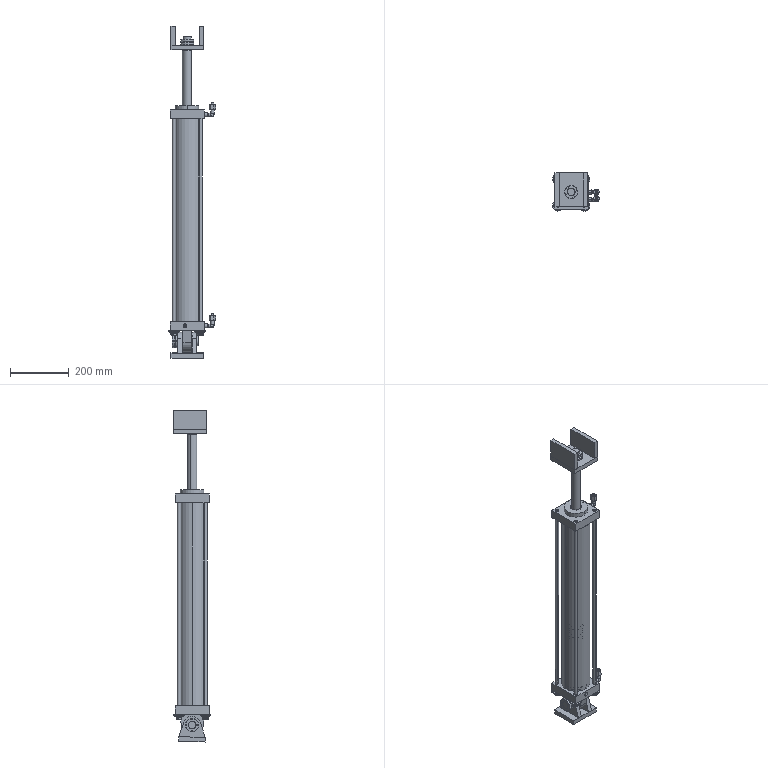Part | SolidWorks | features MirrorCompFeat 2, ReferencePattern 2 | 31 solids | 786 faces | box 159.892 x 128.5 x 1129 mm | volume 3522058 mm3 | cylinder 300 | plane 289 | cone 171 | torus 18 | sphere 6 | spline 2 | commonest cylinder face diameters 3.2 x32 6 x25 90 x18 12.5 x16 45 x16 4 x12